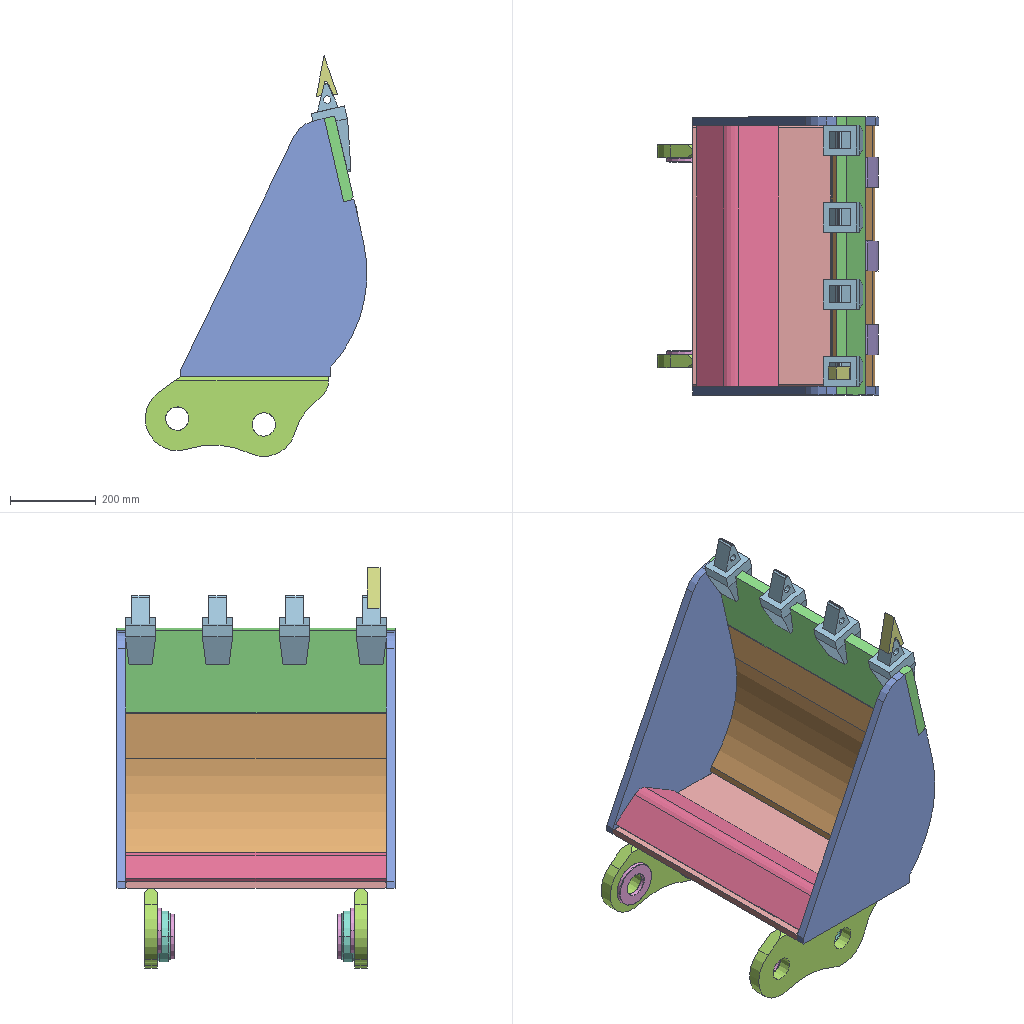Assembly | SolidWorks | 11 different items | 22 placed | box 518 x 650 x 936 mm
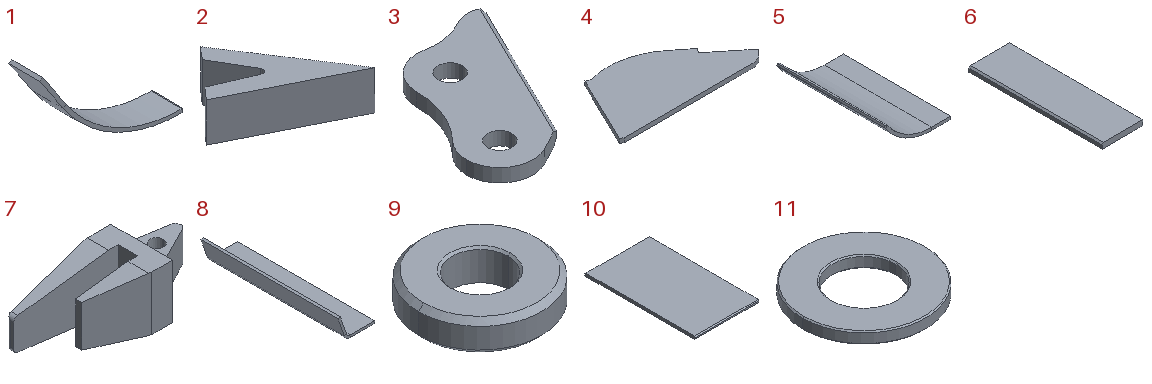Parts list (item | quantity | size | volume | features):
1 | x3 | 325.308 x 70 x 227.668 mm | 230832 mm3 | features FlatPattern 1, SM3dBend 1, SMBaseFlange 1, SheetMetal 1
2 | x1 | 85.955 x 80.416 x 30 mm | 54551 mm3 | features SavedExtBody 1
3 | x2 | 318.374 x 359.351 x 30 mm | 1666573 mm3 | features Chamfer 1, Extrusion 1
4 | x2 | 689.12 x 326 x 20 mm | 3074154 mm3 | features Extrusion 1
5 | x1 | 375.791 x 610 x 155.275 mm | 4096516 mm3 | features Chamfer 2, FlatPattern 1, SM3dBend 1, SMBaseFlange 1, SheetMetal 1
6 | x1 | 200 x 650 x 25 mm | 3229200 mm3 | features Chamfer 1, Extrusion 1
7 | x4 | 213 x 80 x 70 mm | 410977 mm3 | features ICE 2, Extrusion 1, HoleWzd 1
8 | x1 | 163.637 x 610 x 102.048 mm | 1357250 mm3 | features FlatPattern 1, SM3dBend 1, SMBaseFlange 1, SheetMetal 1
9 | x2 | 120 x 120 x 30 mm | 258500 mm3 | features Chamfer 2, Extrusion 1
10 | x1 | 350 x 610 x 16 mm | 3398500 mm3 | features Chamfer 1, Extrusion 1
11 | x4 | 106 x 106 x 10 mm | 63983 mm3 | features Chamfer 1, Extrusion 1
Mates (type | each side: item.copy, entity, surface, feature):
Coincident | 10.1 face plane Boss-Extrude1 | 4.1 face plane Boss-Extrude1 | 3 times
Coincident | 10.1 face plane Boss-Extrude1 | 3.1 face plane Boss-Extrude1
DistanceDim | 4.1 face plane Boss-Extrude1 | 3.1 face plane Boss-Extrude1
Coincident | 10.1 face plane Boss-Extrude1 | 3.1 edge
Coincident | 11.1 face plane Boss-Extrude1 | 9.1 face plane Boss-Extrude1
Concentric | 11.1 face cylinder Boss-Extrude1 | 9.1 face cylinder Boss-Extrude1
Coincident | 3.1 face plane Boss-Extrude1 | 9.1 face plane Boss-Extrude1
Concentric | 3.1 face cylinder Boss-Extrude1 | 9.1 face cylinder Boss-Extrude1
Coincident | 3.1 face plane Boss-Extrude1 | 11.2 face plane Boss-Extrude1
Concentric | 3.1 face cylinder Boss-Extrude1 | 11.2 face cylinder Boss-Extrude1
Concentric | 4.1 face cylinder Boss-Extrude1 | 5.1 face cylinder Sketch Bend1
Coincident | 4.2 face plane Boss-Extrude1 | 5.1 face plane Base-Flange1
Coincident | 10.1 face plane Boss-Extrude1 | 5.1 edge
Concentric | 5.1 face cylinder Sketch Bend1 | 1.1 face cylinder Sketch Bend1
Coincident | 10.1 face plane Boss-Extrude1 | 1.1 edge
DistanceDim | 1.1 face plane Sketch Bend1 | 4.1 face plane Boss-Extrude1
Coincident | 4.1 face plane Boss-Extrude1 | 6.1 face plane Boss-Extrude1
Coincident | 4.2 face plane Boss-Extrude1 | 6.1 face plane Boss-Extrude1 | 2 times
Coincident | 10.1 face plane Boss-Extrude1 | 8.1 edge | 2 times
Coincident | 4.1 face plane Boss-Extrude1 | 8.1 face plane Base-Flange1
Coincident | 4.1 vertex | 8.1 edge
Coincident | 6.1 face plane Boss-Extrude1 | 7.1 face plane Cut-Extrude1 | 3 times
Coincident | 4.2 face plane Boss-Extrude1 | 7.1 face plane Boss-Extrude1
Coincident | 7.2 face plane Boss-Extrude2 | 2.1 face plane Base Body-Bucket-1 | 2 times
Coincident | 7.2 edge | 2.1 face cylinder Base Body-Bucket-1